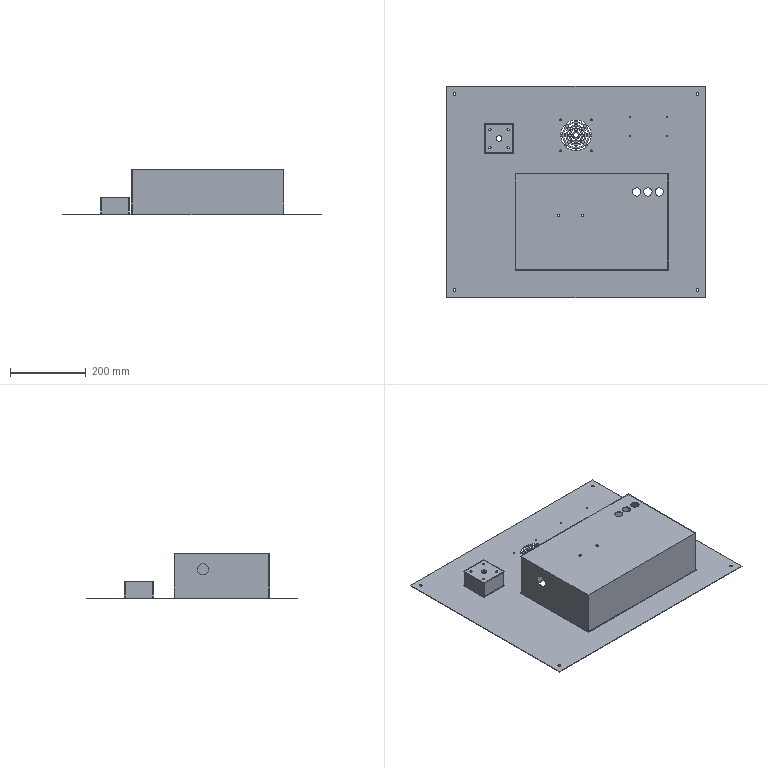Part | STEP file | 09-18 closing plate B | 2 solids | 270 faces | box 683 x 558 x 121.5 mm | volume 815464 mm3 | cylinder 204 | plane 50 | spline 16 | commonest cylinder face diameters 5 x84 7 x12 1.473 x8 3.3 x8 4.473 x8 4.5 x8